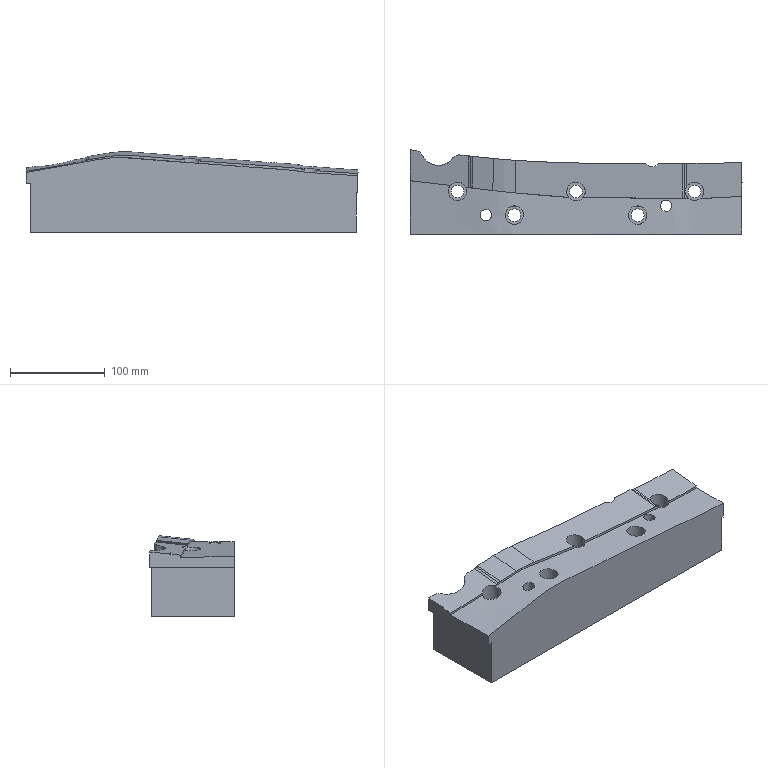Part | NX | features solid 2 | 1 solid | 56 faces | box 350 x 88.874 x 84.892 mm | volume 1743499 mm3 | plane 20 | spline 19 | cylinder 17 | commonest cylinder face diameters 13.5 x5 19.5 x5 10 x4 12 x2 194.4 x1